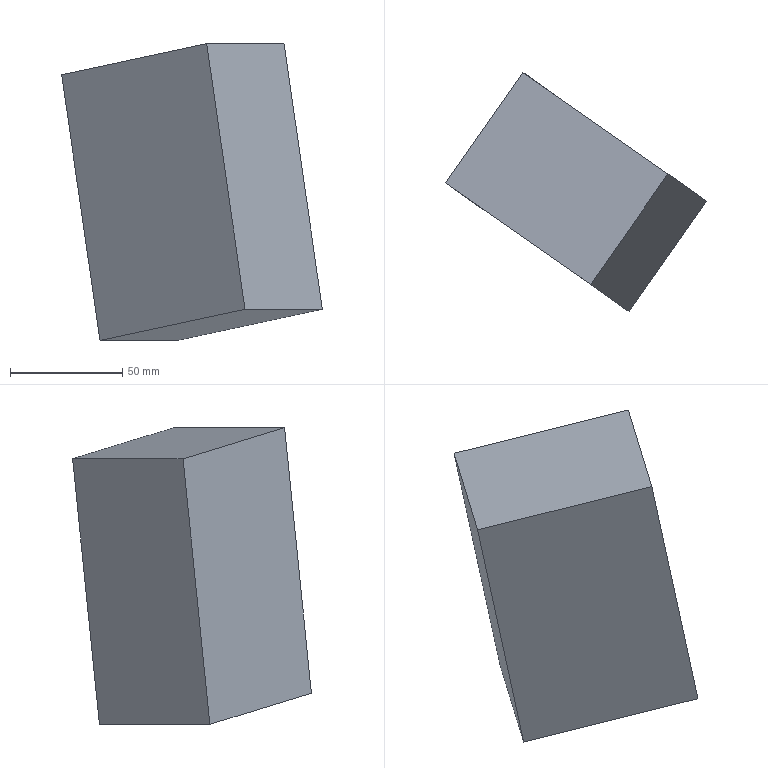Part | NX | features solid 2 | 1 solid | 6 faces | box 116.02 x 106.29 x 132.069 mm | volume 576000 mm3 | plane 6
STEP:
#1=CARTESIAN_POINT('',(201.489,664.627,-88.675));
#2=VERTEX_POINT('',#1);
#3=CARTESIAN_POINT('',(136.952,709.816,-102.567));
#4=VERTEX_POINT('',#3);
#5=CARTESIAN_POINT('',(201.489,664.627,-88.675));
#6=DIRECTION('',(-0.8067,0.5649,-0.1736));
#7=VECTOR('',#6,1000.);
#8=LINE('',#5,#7);
#9=EDGE_CURVE('',#2,#4,#8,.T.);
#10=ORIENTED_EDGE('',*,*,#9,.T.);
#11=CARTESIAN_POINT('',(102.537,660.667,-102.567));
#12=VERTEX_POINT('',#11);
#13=CARTESIAN_POINT('',(96.802,652.476,-102.567));
#14=DIRECTION('',(0.5736,0.8192,0.));
#15=VECTOR('',#14,1000.);
#16=LINE('',#13,#15);
#17=EDGE_CURVE('',#12,#4,#16,.T.);
#18=ORIENTED_EDGE('',*,*,#17,.F.);
#19=CARTESIAN_POINT('',(167.074,615.478,-88.675));
#20=VERTEX_POINT('',#19);
#21=CARTESIAN_POINT('',(167.074,615.478,-88.675));
#22=DIRECTION('',(-0.8067,0.5649,-0.1736));
#23=VECTOR('',#22,1000.);
#24=LINE('',#21,#23);
#25=EDGE_CURVE('',#20,#12,#24,.T.);
#26=ORIENTED_EDGE('',*,*,#25,.F.);
#27=CARTESIAN_POINT('',(161.338,607.287,-88.675));
#28=DIRECTION('',(0.5736,0.8192,0.));
#29=VECTOR('',#28,1000.);
#30=LINE('',#27,#29);
#31=EDGE_CURVE('',#20,#2,#30,.T.);
#32=ORIENTED_EDGE('',*,*,#31,.T.);
#33=EDGE_LOOP('',(#10,#18,#26,#32));
#34=FACE_BOUND('',#33,.T.);
#35=CARTESIAN_POINT('',(161.338,607.287,-88.675));
#36=DIRECTION('',(0.1422,-0.0996,-0.9848));
#37=DIRECTION('',(-0.8067,0.5649,-0.1736));
#38=AXIS2_PLACEMENT_3D('',#35,#36,#37);
#39=PLANE('',#38);
#40=ADVANCED_FACE('',(#34),#39,.F.);
#41=ORIENTED_EDGE('',*,*,#17,.T.);
#42=CARTESIAN_POINT('',(154.021,697.864,-220.744));
#43=VERTEX_POINT('',#42);
#44=CARTESIAN_POINT('',(137.663,709.318,-107.491));
#45=DIRECTION('',(-0.1422,0.0996,0.9848));
#46=VECTOR('',#45,1000.);
#47=LINE('',#44,#46);
#48=EDGE_CURVE('',#4,#43,#47,.F.);
#49=ORIENTED_EDGE('',*,*,#48,.T.);
#50=CARTESIAN_POINT('',(119.607,648.715,-220.744));
#51=VERTEX_POINT('',#50);
#52=CARTESIAN_POINT('',(113.871,640.524,-220.744));
#53=DIRECTION('',(-0.5736,-0.8192,0.));
#54=VECTOR('',#53,1000.);
#55=LINE('',#52,#54);
#56=EDGE_CURVE('',#51,#43,#55,.F.);
#57=ORIENTED_EDGE('',*,*,#56,.F.);
#58=CARTESIAN_POINT('',(103.249,660.169,-107.491));
#59=DIRECTION('',(0.1422,-0.0996,-0.9848));
#60=VECTOR('',#59,1000.);
#61=LINE('',#58,#60);
#62=EDGE_CURVE('',#12,#51,#61,.T.);
#63=ORIENTED_EDGE('',*,*,#62,.F.);
#64=EDGE_LOOP('',(#41,#49,#57,#63));
#65=FACE_BOUND('',#64,.T.);
#66=CARTESIAN_POINT('',(97.513,651.978,-107.491));
#67=DIRECTION('',(0.8067,-0.5649,0.1736));
#68=DIRECTION('',(0.1422,-0.0996,-0.9848));
#69=AXIS2_PLACEMENT_3D('',#66,#67,#68);
#70=PLANE('',#69);
#71=ADVANCED_FACE('',(#65),#70,.F.);
#72=ORIENTED_EDGE('',*,*,#56,.T.);
#73=CARTESIAN_POINT('',(218.558,652.675,-206.852));
#74=VERTEX_POINT('',#73);
#75=CARTESIAN_POINT('',(218.558,652.675,-206.852));
#76=DIRECTION('',(0.8067,-0.5649,0.1736));
#77=VECTOR('',#76,1000.);
#78=LINE('',#75,#77);
#79=EDGE_CURVE('',#74,#43,#78,.F.);
#80=ORIENTED_EDGE('',*,*,#79,.F.);
#81=CARTESIAN_POINT('',(184.143,603.526,-206.852));
#82=VERTEX_POINT('',#81);
#83=CARTESIAN_POINT('',(178.407,595.335,-206.852));
#84=DIRECTION('',(-0.5736,-0.8192,0.));
#85=VECTOR('',#84,1000.);
#86=LINE('',#83,#85);
#87=EDGE_CURVE('',#82,#74,#86,.F.);
#88=ORIENTED_EDGE('',*,*,#87,.F.);
#89=CARTESIAN_POINT('',(184.143,603.526,-206.852));
#90=DIRECTION('',(0.8067,-0.5649,0.1736));
#91=VECTOR('',#90,1000.);
#92=LINE('',#89,#91);
#93=EDGE_CURVE('',#82,#51,#92,.F.);
#94=ORIENTED_EDGE('',*,*,#93,.T.);
#95=EDGE_LOOP('',(#72,#80,#88,#94));
#96=FACE_BOUND('',#95,.T.);
#97=CARTESIAN_POINT('',(178.407,595.335,-206.852));
#98=DIRECTION('',(0.1422,-0.0996,-0.9848));
#99=DIRECTION('',(-0.8067,0.5649,-0.1736));
#100=AXIS2_PLACEMENT_3D('',#97,#98,#99);
#101=PLANE('',#100);
#102=ADVANCED_FACE('',(#96),#101,.T.);
#103=ORIENTED_EDGE('',*,*,#79,.T.);
#104=ORIENTED_EDGE('',*,*,#48,.F.);
#105=ORIENTED_EDGE('',*,*,#9,.F.);
#106=CARTESIAN_POINT('',(202.2,664.129,-93.6));
#107=DIRECTION('',(0.1422,-0.0996,-0.9848));
#108=VECTOR('',#107,1000.);
#109=LINE('',#106,#108);
#110=EDGE_CURVE('',#2,#74,#109,.T.);
#111=ORIENTED_EDGE('',*,*,#110,.T.);
#112=EDGE_LOOP('',(#103,#104,#105,#111));
#113=FACE_BOUND('',#112,.T.);
#114=CARTESIAN_POINT('',(202.2,664.129,-93.6));
#115=DIRECTION('',(0.5736,0.8192,0.));
#116=DIRECTION('',(-0.8192,0.5736,0.));
#117=AXIS2_PLACEMENT_3D('',#114,#115,#116);
#118=PLANE('',#117);
#119=ADVANCED_FACE('',(#113),#118,.T.);
#120=ORIENTED_EDGE('',*,*,#25,.T.);
#121=ORIENTED_EDGE('',*,*,#62,.T.);
#122=ORIENTED_EDGE('',*,*,#93,.F.);
#123=CARTESIAN_POINT('',(167.785,614.98,-93.6));
#124=DIRECTION('',(-0.1422,0.0996,0.9848));
#125=VECTOR('',#124,1000.);
#126=LINE('',#123,#125);
#127=EDGE_CURVE('',#82,#20,#126,.T.);
#128=ORIENTED_EDGE('',*,*,#127,.T.);
#129=EDGE_LOOP('',(#120,#121,#122,#128));
#130=FACE_BOUND('',#129,.T.);
#131=CARTESIAN_POINT('',(167.785,614.98,-93.6));
#132=DIRECTION('',(0.5736,0.8192,0.));
#133=DIRECTION('',(-0.8192,0.5736,0.));
#134=AXIS2_PLACEMENT_3D('',#131,#132,#133);
#135=PLANE('',#134);
#136=ADVANCED_FACE('',(#130),#135,.F.);
#137=ORIENTED_EDGE('',*,*,#31,.F.);
#138=ORIENTED_EDGE('',*,*,#127,.F.);
#139=ORIENTED_EDGE('',*,*,#87,.T.);
#140=ORIENTED_EDGE('',*,*,#110,.F.);
#141=EDGE_LOOP('',(#137,#138,#139,#140));
#142=FACE_BOUND('',#141,.T.);
#143=CARTESIAN_POINT('',(162.049,606.789,-93.6));
#144=DIRECTION('',(0.8067,-0.5649,0.1736));
#145=DIRECTION('',(0.1422,-0.0996,-0.9848));
#146=AXIS2_PLACEMENT_3D('',#143,#144,#145);
#147=PLANE('',#146);
#148=ADVANCED_FACE('',(#142),#147,.T.);
#149=CLOSED_SHELL('',(#40,#71,#102,#119,#136,#148));
#150=MANIFOLD_SOLID_BREP('',#149);
#151=(LENGTH_UNIT()NAMED_UNIT(*)SI_UNIT(.MILLI.,.METRE.));
#152=UNCERTAINTY_MEASURE_WITH_UNIT(LENGTH_MEASURE(0.00001),#151,'','');
#153=(NAMED_UNIT(*)PLANE_ANGLE_UNIT()SI_UNIT($,.RADIAN.));
#154=(NAMED_UNIT(*)SI_UNIT($,.STERADIAN.)SOLID_ANGLE_UNIT());
#155=(GEOMETRIC_REPRESENTATION_CONTEXT(3)GLOBAL_UNCERTAINTY_ASSIGNED_CONTEXT((#152))GLOBAL_UNIT_ASSIGNED_CONTEXT((#151,#153,#154))REPRESENTATION_CONTEXT('',''));
#156=ADVANCED_BREP_SHAPE_REPRESENTATION('',(#150),#155);